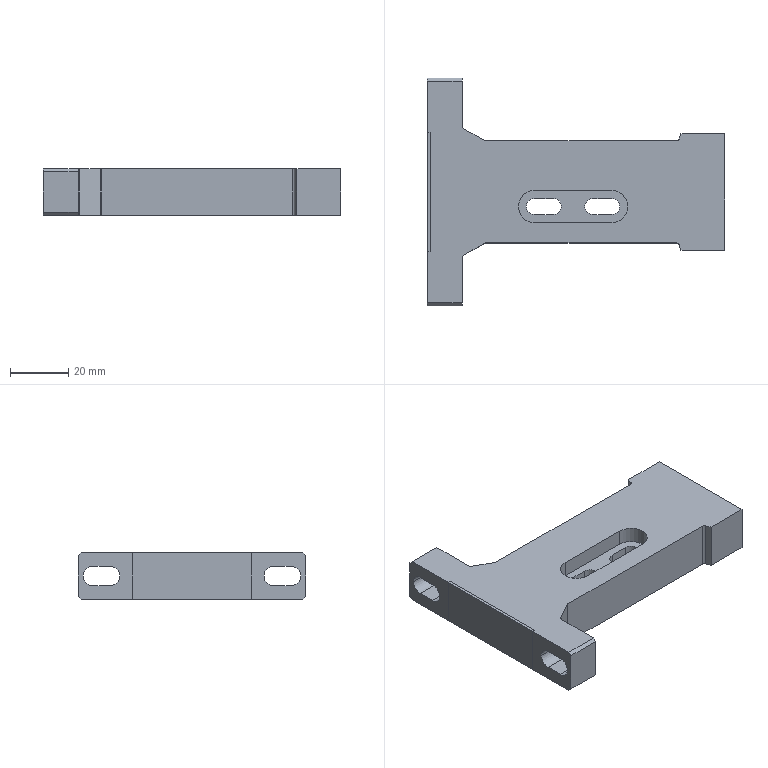NC program | NX | posted with a generic post | part box 102 x 78 x 16 mm
Whole program:
N10 G17 G21 G94 G90
(DRILLING_COPY_1 , TOOL : D6A45)
N12 T07 M6
N14 G54
N16 G17 G0 G90 X-12.5 Y0. B0. C0. S5000 M3
N18 G43 Z30. H7
N20 G94 G81 G98 Z-2.6 F250. R3.
N22 X12.5
N24 G80
N26 G0 X12.5 Y0. Z30.
(DRILLING_COPY_1_COPY , TOOL : D6A45)
N28 X-4.
N30 G81 Z-2.1 F250. R3.
N32 X4.
N34 G80
N36 G0 X4. Y0. Z30.
N38 M5
(DRILLING_COPY , TOOL : 5.0ZT)
N40 T14 M6
N42 G54
N44 G17 G0 G90 X12.5 Y0. B0. C0. S2000 M3
N46 G43 Z30. H14
N48 G94 G83 G98 Z-16.262 F150. Q2. R3.
N50 X-12.5
N52 G80
N54 G0 X-12.5 Y0. Z30.
N56 M5
(DRILLING_COPY_COPY_1 , TOOL : 3.8ZT)
N58 T13 M6
N60 G54
N62 G17 G0 G90 X-4. Y0. B0. C0. S2000 M3
N64 G43 Z30. H13
N66 G94 G83 G98 Z-14.542 F150. Q2. R3.
N68 X4.
N70 G80
N72 G0 X4. Y0. Z30.
N74 M5
(DRILLING_COPY_COPY_1_COPY , TOOL : 4.0JD)
N76 T12 M6
N78 G54
N80 G17 G0 G90 X-4. Y0. B0. C0. S1000 M3
N82 G43 Z30. H12
N84 G94 G85 G98 Z-13.4 F50. R3.
N86 X4.
N88 G80
N90 G0 X4. Y0. Z30.
N92 M5
N94 M2